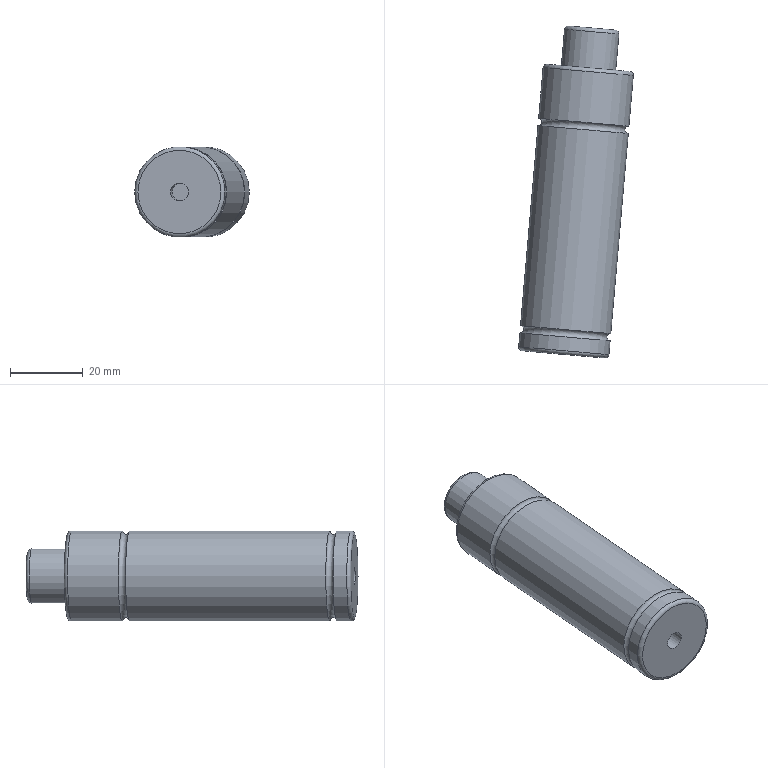Part | NX | features 1 2 | 1 solid | 17 faces | box 31.524 x 91.23 x 24.9 mm | volume 40004 mm3 | cylinder 6 | torus 5 | plane 4 | cone 2 | commonest cylinder face diameters 24.9 x3 2 x1 4.9 x1 15 x1
STEP:
#1=CARTESIAN_POINT('',(310.52,-35.699,-85.));
#2=VERTEX_POINT('',#1);
#3=CARTESIAN_POINT('',(298.118,-34.614,-85.));
#4=DIRECTION('',(0.08716,0.9962,0.));
#5=DIRECTION('',(0.9962,-0.08716,0.));
#6=AXIS2_PLACEMENT_3D('',#3,#4,#5);
#7=CIRCLE('',#6,12.45);
#8=EDGE_CURVE('',#2,#2,#7,.T.);
#9=ORIENTED_EDGE('',*,*,#8,.T.);
#10=EDGE_LOOP('',(#9));
#11=FACE_BOUND('',#10,.T.);
#12=CARTESIAN_POINT('',(310.695,-33.707,-85.));
#13=VERTEX_POINT('',#12);
#14=CARTESIAN_POINT('',(298.292,-32.622,-85.));
#15=DIRECTION('',(0.08716,0.9962,0.));
#16=DIRECTION('',(0.9962,-0.08716,0.));
#17=AXIS2_PLACEMENT_3D('',#14,#15,#16);
#18=CIRCLE('',#17,12.45);
#19=EDGE_CURVE('',#13,#13,#18,.T.);
#20=ORIENTED_EDGE('',*,*,#19,.F.);
#21=EDGE_LOOP('',(#20));
#22=FACE_BOUND('',#21,.T.);
#23=CARTESIAN_POINT('',(298.205,-33.618,-85.));
#24=DIRECTION('',(0.08716,0.9962,0.));
#25=DIRECTION('',(0.,0.,1.));
#26=AXIS2_PLACEMENT_3D('',#23,#24,#25);
#27=TOROIDAL_SURFACE('',#26,12.45,1.);
#28=ADVANCED_FACE('',(#11,#22),#27,.F.);
#29=CARTESIAN_POINT('',(305.709,-90.689,-85.));
#30=VERTEX_POINT('',#29);
#31=CARTESIAN_POINT('',(293.307,-89.604,-85.));
#32=DIRECTION('',(0.08716,0.9962,0.));
#33=DIRECTION('',(0.9962,-0.08716,0.));
#34=AXIS2_PLACEMENT_3D('',#31,#32,#33);
#35=CIRCLE('',#34,12.45);
#36=EDGE_CURVE('',#30,#30,#35,.T.);
#37=ORIENTED_EDGE('',*,*,#36,.F.);
#38=EDGE_LOOP('',(#37));
#39=FACE_BOUND('',#38,.T.);
#40=CARTESIAN_POINT('',(305.535,-92.682,-85.));
#41=VERTEX_POINT('',#40);
#42=CARTESIAN_POINT('',(293.132,-91.597,-85.));
#43=DIRECTION('',(-0.08716,-0.9962,0.));
#44=DIRECTION('',(0.9962,-0.08716,0.));
#45=AXIS2_PLACEMENT_3D('',#42,#43,#44);
#46=CIRCLE('',#45,12.45);
#47=EDGE_CURVE('',#41,#41,#46,.T.);
#48=ORIENTED_EDGE('',*,*,#47,.F.);
#49=EDGE_LOOP('',(#48));
#50=FACE_BOUND('',#49,.T.);
#51=CARTESIAN_POINT('',(293.219,-90.601,-85.));
#52=DIRECTION('',(0.08716,0.9962,0.));
#53=DIRECTION('',(0.,0.,1.));
#54=AXIS2_PLACEMENT_3D('',#51,#52,#53);
#55=TOROIDAL_SURFACE('',#54,12.45,1.);
#56=ADVANCED_FACE('',(#39,#50),#55,.F.);
#57=CARTESIAN_POINT('',(311.915,-19.76,-85.));
#58=VERTEX_POINT('',#57);
#59=CARTESIAN_POINT('',(299.512,-18.675,-85.));
#60=DIRECTION('',(0.08716,0.9962,0.));
#61=DIRECTION('',(0.9962,-0.08716,0.));
#62=AXIS2_PLACEMENT_3D('',#59,#60,#61);
#63=CIRCLE('',#62,12.45);
#64=EDGE_CURVE('',#58,#58,#63,.T.);
#65=ORIENTED_EDGE('',*,*,#64,.T.);
#66=EDGE_LOOP('',(#65));
#67=FACE_BOUND('',#66,.T.);
#68=CARTESIAN_POINT('',(311.006,-18.677,-85.));
#69=VERTEX_POINT('',#68);
#70=CARTESIAN_POINT('',(299.599,-17.679,-85.));
#71=DIRECTION('',(0.08716,0.9962,0.));
#72=DIRECTION('',(0.9962,-0.08716,0.));
#73=AXIS2_PLACEMENT_3D('',#70,#71,#72);
#74=CIRCLE('',#73,11.45);
#75=EDGE_CURVE('',#69,#69,#74,.T.);
#76=ORIENTED_EDGE('',*,*,#75,.F.);
#77=EDGE_LOOP('',(#76));
#78=FACE_BOUND('',#77,.T.);
#79=CARTESIAN_POINT('',(299.512,-18.675,-85.));
#80=DIRECTION('',(0.08716,0.9962,0.));
#81=DIRECTION('',(0.,0.,1.));
#82=AXIS2_PLACEMENT_3D('',#79,#80,#81);
#83=TOROIDAL_SURFACE('',#82,11.45,1.);
#84=ADVANCED_FACE('',(#67,#78),#83,.T.);
#85=ORIENTED_EDGE('',*,*,#19,.T.);
#86=EDGE_LOOP('',(#85));
#87=FACE_BOUND('',#86,.T.);
#88=ORIENTED_EDGE('',*,*,#64,.F.);
#89=EDGE_LOOP('',(#88));
#90=FACE_BOUND('',#89,.T.);
#91=CARTESIAN_POINT('',(298.902,-25.649,-85.));
#92=DIRECTION('',(-0.08716,-0.9962,0.));
#93=DIRECTION('',(0.,0.,-1.));
#94=AXIS2_PLACEMENT_3D('',#91,#92,#93);
#95=CYLINDRICAL_SURFACE('',#94,12.45);
#96=ADVANCED_FACE('',(#87,#90),#95,.T.);
#97=ORIENTED_EDGE('',*,*,#36,.T.);
#98=EDGE_LOOP('',(#97));
#99=FACE_BOUND('',#98,.T.);
#100=ORIENTED_EDGE('',*,*,#8,.F.);
#101=EDGE_LOOP('',(#100));
#102=FACE_BOUND('',#101,.T.);
#103=CARTESIAN_POINT('',(295.459,-64.998,-85.));
#104=DIRECTION('',(-0.08716,-0.9962,0.));
#105=DIRECTION('',(0.,0.,-1.));
#106=AXIS2_PLACEMENT_3D('',#103,#104,#105);
#107=CYLINDRICAL_SURFACE('',#106,12.45);
#108=ADVANCED_FACE('',(#99,#102),#107,.T.);
#109=CARTESIAN_POINT('',(304.12,-97.376,-85.));
#110=VERTEX_POINT('',#109);
#111=CARTESIAN_POINT('',(292.714,-96.378,-85.));
#112=DIRECTION('',(0.08716,0.9962,0.));
#113=DIRECTION('',(0.9962,-0.08716,0.));
#114=AXIS2_PLACEMENT_3D('',#111,#112,#113);
#115=CIRCLE('',#114,11.45);
#116=EDGE_CURVE('',#110,#110,#115,.T.);
#117=ORIENTED_EDGE('',*,*,#116,.T.);
#118=EDGE_LOOP('',(#117));
#119=FACE_BOUND('',#118,.T.);
#120=CARTESIAN_POINT('',(305.204,-96.467,-85.));
#121=VERTEX_POINT('',#120);
#122=CARTESIAN_POINT('',(292.801,-95.382,-85.));
#123=DIRECTION('',(0.08716,0.9962,0.));
#124=DIRECTION('',(0.9962,-0.08716,0.));
#125=AXIS2_PLACEMENT_3D('',#122,#123,#124);
#126=CIRCLE('',#125,12.45);
#127=EDGE_CURVE('',#121,#121,#126,.T.);
#128=ORIENTED_EDGE('',*,*,#127,.F.);
#129=EDGE_LOOP('',(#128));
#130=FACE_BOUND('',#129,.T.);
#131=CARTESIAN_POINT('',(292.801,-95.382,-85.));
#132=DIRECTION('',(0.08716,0.9962,0.));
#133=DIRECTION('',(0.,0.,1.));
#134=AXIS2_PLACEMENT_3D('',#131,#132,#133);
#135=TOROIDAL_SURFACE('',#134,11.45,1.);
#136=ADVANCED_FACE('',(#119,#130),#135,.T.);
#137=ORIENTED_EDGE('',*,*,#127,.T.);
#138=EDGE_LOOP('',(#137));
#139=FACE_BOUND('',#138,.T.);
#140=ORIENTED_EDGE('',*,*,#47,.T.);
#141=EDGE_LOOP('',(#140));
#142=FACE_BOUND('',#141,.T.);
#143=CARTESIAN_POINT('',(295.459,-64.998,-85.));
#144=DIRECTION('',(-0.08716,-0.9962,0.));
#145=DIRECTION('',(0.,0.,-1.));
#146=AXIS2_PLACEMENT_3D('',#143,#144,#145);
#147=CYLINDRICAL_SURFACE('',#146,12.45);
#148=ADVANCED_FACE('',(#139,#142),#147,.T.);
#149=CARTESIAN_POINT('',(307.942,-8.371,-85.));
#150=VERTEX_POINT('',#149);
#151=CARTESIAN_POINT('',(300.471,-7.717,-85.));
#152=DIRECTION('',(0.08716,0.9962,0.));
#153=DIRECTION('',(0.9962,-0.08716,0.));
#154=AXIS2_PLACEMENT_3D('',#151,#152,#153);
#155=CIRCLE('',#154,7.5);
#156=EDGE_CURVE('',#150,#150,#155,.T.);
#157=ORIENTED_EDGE('',*,*,#156,.T.);
#158=EDGE_LOOP('',(#157));
#159=FACE_BOUND('',#158,.T.);
#160=CARTESIAN_POINT('',(307.033,-7.287,-85.));
#161=VERTEX_POINT('',#160);
#162=CARTESIAN_POINT('',(300.558,-6.721,-85.));
#163=DIRECTION('',(0.08716,0.9962,0.));
#164=DIRECTION('',(0.9962,-0.08716,0.));
#165=AXIS2_PLACEMENT_3D('',#162,#163,#164);
#166=CIRCLE('',#165,6.5);
#167=EDGE_CURVE('',#161,#161,#166,.T.);
#168=ORIENTED_EDGE('',*,*,#167,.F.);
#169=EDGE_LOOP('',(#168));
#170=FACE_BOUND('',#169,.T.);
#171=CARTESIAN_POINT('',(300.471,-7.717,-85.));
#172=DIRECTION('',(0.08716,0.9962,0.));
#173=DIRECTION('',(0.,0.,1.));
#174=AXIS2_PLACEMENT_3D('',#171,#172,#173);
#175=TOROIDAL_SURFACE('',#174,6.5,1.);
#176=ADVANCED_FACE('',(#159,#170),#175,.T.);
#177=CARTESIAN_POINT('',(307.071,-18.333,-85.));
#178=VERTEX_POINT('',#177);
#179=CARTESIAN_POINT('',(299.599,-17.679,-85.));
#180=DIRECTION('',(-0.08716,-0.9962,0.));
#181=DIRECTION('',(0.9962,-0.08716,0.));
#182=AXIS2_PLACEMENT_3D('',#179,#180,#181);
#183=CIRCLE('',#182,7.5);
#184=EDGE_CURVE('',#178,#178,#183,.T.);
#185=ORIENTED_EDGE('',*,*,#184,.F.);
#186=EDGE_LOOP('',(#185));
#187=FACE_BOUND('',#186,.T.);
#188=ORIENTED_EDGE('',*,*,#156,.F.);
#189=EDGE_LOOP('',(#188));
#190=FACE_BOUND('',#189,.T.);
#191=CARTESIAN_POINT('',(300.035,-12.698,-85.));
#192=DIRECTION('',(-0.08716,-0.9962,0.));
#193=DIRECTION('',(0.,0.,-1.));
#194=AXIS2_PLACEMENT_3D('',#191,#192,#193);
#195=CYLINDRICAL_SURFACE('',#194,7.5);
#196=ADVANCED_FACE('',(#187,#190),#195,.T.);
#197=CARTESIAN_POINT('',(302.55,-6.895,-85.));
#198=VERTEX_POINT('',#197);
#199=CARTESIAN_POINT('',(300.558,-6.721,-85.));
#200=DIRECTION('',(-0.08716,-0.9962,0.));
#201=DIRECTION('',(0.9962,-0.08716,0.));
#202=AXIS2_PLACEMENT_3D('',#199,#200,#201);
#203=CIRCLE('',#202,2.);
#204=EDGE_CURVE('',#198,#198,#203,.T.);
#205=ORIENTED_EDGE('',*,*,#204,.F.);
#206=EDGE_LOOP('',(#205));
#207=FACE_BOUND('',#206,.T.);
#208=CARTESIAN_POINT('',(301.403,-8.534,-85.));
#209=VERTEX_POINT('',#208);
#210=CARTESIAN_POINT('',(300.407,-8.446,-85.));
#211=DIRECTION('',(0.08716,0.9962,0.));
#212=DIRECTION('',(0.9962,-0.08716,0.));
#213=AXIS2_PLACEMENT_3D('',#210,#211,#212);
#214=CIRCLE('',#213,1.);
#215=EDGE_CURVE('',#209,#209,#214,.T.);
#216=ORIENTED_EDGE('',*,*,#215,.F.);
#217=EDGE_LOOP('',(#216));
#218=FACE_BOUND('',#217,.T.);
#219=CARTESIAN_POINT('',(300.482,-7.584,-85.));
#220=DIRECTION('',(0.08716,0.9962,0.));
#221=DIRECTION('',(0.,0.,1.));
#222=AXIS2_PLACEMENT_3D('',#219,#220,#221);
#223=CONICAL_SURFACE('',#222,1.5,0.5236);
#224=ADVANCED_FACE('',(#207,#218),#223,.F.);
#225=ORIENTED_EDGE('',*,*,#215,.T.);
#226=EDGE_LOOP('',(#225));
#227=FACE_BOUND('',#226,.T.);
#228=CARTESIAN_POINT('',(301.075,-12.287,-85.));
#229=VERTEX_POINT('',#228);
#230=CARTESIAN_POINT('',(300.079,-12.2,-85.));
#231=DIRECTION('',(0.08716,0.9962,0.));
#232=DIRECTION('',(0.9962,-0.08716,0.));
#233=AXIS2_PLACEMENT_3D('',#230,#231,#232);
#234=CIRCLE('',#233,1.);
#235=EDGE_CURVE('',#229,#229,#234,.T.);
#236=ORIENTED_EDGE('',*,*,#235,.F.);
#237=EDGE_LOOP('',(#236));
#238=FACE_BOUND('',#237,.T.);
#239=CARTESIAN_POINT('',(300.243,-10.323,-85.));
#240=DIRECTION('',(-0.08716,-0.9962,0.));
#241=DIRECTION('',(0.,0.,-1.));
#242=AXIS2_PLACEMENT_3D('',#239,#240,#241);
#243=CYLINDRICAL_SURFACE('',#242,1.);
#244=ADVANCED_FACE('',(#227,#238),#243,.F.);
#245=CARTESIAN_POINT('',(300.035,-12.698,-85.));
#246=VERTEX_POINT('',#245);
#247=VERTEX_LOOP('',#246);
#248=FACE_BOUND('',#247,.T.);
#249=ORIENTED_EDGE('',*,*,#235,.T.);
#250=EDGE_LOOP('',(#249));
#251=FACE_BOUND('',#250,.T.);
#252=CARTESIAN_POINT('',(300.057,-12.449,-85.));
#253=DIRECTION('',(0.08716,0.9962,0.));
#254=DIRECTION('',(0.,0.,1.));
#255=AXIS2_PLACEMENT_3D('',#252,#253,#254);
#256=CONICAL_SURFACE('',#255,0.5,1.107);
#257=ADVANCED_FACE('',(#248,#251),#256,.F.);
#258=CARTESIAN_POINT('',(295.634,-91.113,-85.));
#259=VERTEX_POINT('',#258);
#260=CARTESIAN_POINT('',(293.193,-90.899,-85.));
#261=DIRECTION('',(-0.08716,-0.9962,0.));
#262=DIRECTION('',(0.9962,-0.08716,0.));
#263=AXIS2_PLACEMENT_3D('',#260,#261,#262);
#264=CIRCLE('',#263,2.45);
#265=EDGE_CURVE('',#259,#259,#264,.T.);
#266=ORIENTED_EDGE('',*,*,#265,.F.);
#267=EDGE_LOOP('',(#266));
#268=FACE_BOUND('',#267,.T.);
#269=CARTESIAN_POINT('',(295.155,-96.592,-85.));
#270=VERTEX_POINT('',#269);
#271=CARTESIAN_POINT('',(292.714,-96.378,-85.));
#272=DIRECTION('',(0.08716,0.9962,0.));
#273=DIRECTION('',(0.9962,-0.08716,0.));
#274=AXIS2_PLACEMENT_3D('',#271,#272,#273);
#275=CIRCLE('',#274,2.45);
#276=EDGE_CURVE('',#270,#270,#275,.T.);
#277=ORIENTED_EDGE('',*,*,#276,.F.);
#278=EDGE_LOOP('',(#277));
#279=FACE_BOUND('',#278,.T.);
#280=CARTESIAN_POINT('',(292.714,-96.378,-85.));
#281=DIRECTION('',(-0.08716,-0.9962,0.));
#282=DIRECTION('',(0.,0.,-1.));
#283=AXIS2_PLACEMENT_3D('',#280,#281,#282);
#284=CYLINDRICAL_SURFACE('',#283,2.45);
#285=ADVANCED_FACE('',(#268,#279),#284,.F.);
#286=ORIENTED_EDGE('',*,*,#265,.T.);
#287=EDGE_LOOP('',(#286));
#288=FACE_BOUND('',#287,.T.);
#289=CARTESIAN_POINT('',(293.193,-90.899,-85.));
#290=DIRECTION('',(-0.08716,-0.9962,0.));
#291=DIRECTION('',(0.,0.,-1.));
#292=AXIS2_PLACEMENT_3D('',#289,#290,#291);
#293=PLANE('',#292);
#294=ADVANCED_FACE('',(#288),#293,.T.);
#295=ORIENTED_EDGE('',*,*,#204,.T.);
#296=EDGE_LOOP('',(#295));
#297=FACE_BOUND('',#296,.T.);
#298=ORIENTED_EDGE('',*,*,#167,.T.);
#299=EDGE_LOOP('',(#298));
#300=FACE_BOUND('',#299,.T.);
#301=CARTESIAN_POINT('',(303.796,-7.004,-85.));
#302=DIRECTION('',(0.08716,0.9962,0.));
#303=DIRECTION('',(0.,0.,1.));
#304=AXIS2_PLACEMENT_3D('',#301,#302,#303);
#305=PLANE('',#304);
#306=ADVANCED_FACE('',(#297,#300),#305,.T.);
#307=ORIENTED_EDGE('',*,*,#276,.T.);
#308=EDGE_LOOP('',(#307));
#309=FACE_BOUND('',#308,.T.);
#310=ORIENTED_EDGE('',*,*,#116,.F.);
#311=EDGE_LOOP('',(#310));
#312=FACE_BOUND('',#311,.T.);
#313=CARTESIAN_POINT('',(298.417,-96.877,-85.));
#314=DIRECTION('',(-0.08716,-0.9962,0.));
#315=DIRECTION('',(0.9962,-0.08716,0.));
#316=AXIS2_PLACEMENT_3D('',#313,#314,#315);
#317=PLANE('',#316);
#318=ADVANCED_FACE('',(#309,#312),#317,.T.);
#319=ORIENTED_EDGE('',*,*,#184,.T.);
#320=EDGE_LOOP('',(#319));
#321=FACE_BOUND('',#320,.T.);
#322=ORIENTED_EDGE('',*,*,#75,.T.);
#323=EDGE_LOOP('',(#322));
#324=FACE_BOUND('',#323,.T.);
#325=CARTESIAN_POINT('',(305.302,-18.178,-85.));
#326=DIRECTION('',(0.08716,0.9962,0.));
#327=DIRECTION('',(0.,0.,1.));
#328=AXIS2_PLACEMENT_3D('',#325,#326,#327);
#329=PLANE('',#328);
#330=ADVANCED_FACE('',(#321,#324),#329,.T.);
#331=CLOSED_SHELL('',(#28,#56,#84,#96,#108,#136,#148,#176,#196,#224,#244,#257,#285,#294,#306,#318,#330));
#332=MANIFOLD_SOLID_BREP('',#331);
#333=(LENGTH_UNIT()NAMED_UNIT(*)SI_UNIT(.MILLI.,.METRE.));
#334=UNCERTAINTY_MEASURE_WITH_UNIT(LENGTH_MEASURE(0.00001),#333,'','');
#335=(NAMED_UNIT(*)PLANE_ANGLE_UNIT()SI_UNIT($,.RADIAN.));
#336=(NAMED_UNIT(*)SI_UNIT($,.STERADIAN.)SOLID_ANGLE_UNIT());
#337=(GEOMETRIC_REPRESENTATION_CONTEXT(3)GLOBAL_UNCERTAINTY_ASSIGNED_CONTEXT((#334))GLOBAL_UNIT_ASSIGNED_CONTEXT((#333,#335,#336))REPRESENTATION_CONTEXT('',''));
#338=ADVANCED_BREP_SHAPE_REPRESENTATION('',(#332),#337);